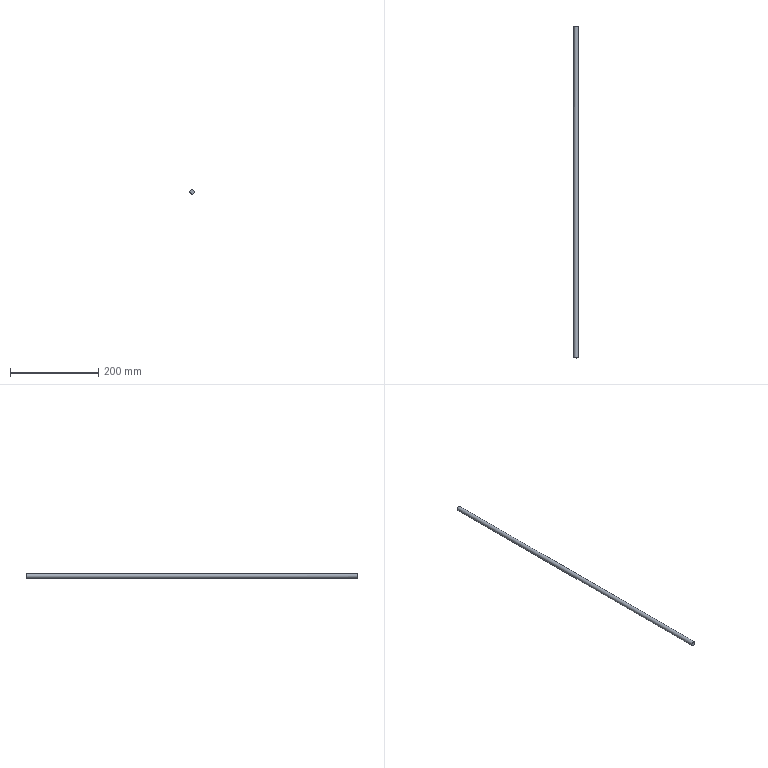Part | NX | features solid 2 | 1 solid | 3 faces | box 10 x 751.5 x 10 mm | volume 59023 mm3 | plane 2 | cylinder 1 | commonest cylinder face diameters 10 x1
STEP:
#1=CARTESIAN_POINT('',(1175.,436.5,-367.));
#2=VERTEX_POINT('',#1);
#3=CARTESIAN_POINT('',(1175.,436.5,-362.));
#4=DIRECTION('',(0.,-1.,0.));
#5=DIRECTION('',(0.,0.,-1.));
#6=AXIS2_PLACEMENT_3D('',#3,#4,#5);
#7=CIRCLE('',#6,5.);
#8=EDGE_CURVE('',#2,#2,#7,.F.);
#9=ORIENTED_EDGE('',*,*,#8,.T.);
#10=EDGE_LOOP('',(#9));
#11=FACE_BOUND('',#10,.T.);
#12=CARTESIAN_POINT('',(1175.,436.5,-362.));
#13=DIRECTION('',(0.,-1.,0.));
#14=DIRECTION('',(0.,0.,1.));
#15=AXIS2_PLACEMENT_3D('',#12,#13,#14);
#16=PLANE('',#15);
#17=ADVANCED_FACE('',(#11),#16,.F.);
#18=CARTESIAN_POINT('',(1170.,-315.,-362.));
#19=VERTEX_POINT('',#18);
#20=CARTESIAN_POINT('',(1175.,-315.,-362.));
#21=DIRECTION('',(0.,1.,0.));
#22=DIRECTION('',(-1.,0.,0.));
#23=AXIS2_PLACEMENT_3D('',#20,#21,#22);
#24=CIRCLE('',#23,5.);
#25=EDGE_CURVE('',#19,#19,#24,.F.);
#26=ORIENTED_EDGE('',*,*,#25,.F.);
#27=EDGE_LOOP('',(#26));
#28=FACE_BOUND('',#27,.T.);
#29=ORIENTED_EDGE('',*,*,#8,.F.);
#30=EDGE_LOOP('',(#29));
#31=FACE_BOUND('',#30,.T.);
#32=CARTESIAN_POINT('',(1175.,-613.5,-362.));
#33=DIRECTION('',(0.,1.,0.));
#34=DIRECTION('',(0.,0.,-1.));
#35=AXIS2_PLACEMENT_3D('',#32,#33,#34);
#36=CYLINDRICAL_SURFACE('',#35,5.);
#37=ADVANCED_FACE('',(#28,#31),#36,.T.);
#38=ORIENTED_EDGE('',*,*,#25,.T.);
#39=EDGE_LOOP('',(#38));
#40=FACE_BOUND('',#39,.T.);
#41=CARTESIAN_POINT('',(1385.,-315.,-350.));
#42=DIRECTION('',(0.,1.,0.));
#43=DIRECTION('',(-1.,0.,0.));
#44=AXIS2_PLACEMENT_3D('',#41,#42,#43);
#45=PLANE('',#44);
#46=ADVANCED_FACE('',(#40),#45,.F.);
#47=CLOSED_SHELL('',(#17,#37,#46));
#48=MANIFOLD_SOLID_BREP('',#47);
#49=(LENGTH_UNIT()NAMED_UNIT(*)SI_UNIT(.MILLI.,.METRE.));
#50=UNCERTAINTY_MEASURE_WITH_UNIT(LENGTH_MEASURE(0.00001),#49,'','');
#51=(NAMED_UNIT(*)PLANE_ANGLE_UNIT()SI_UNIT($,.RADIAN.));
#52=(NAMED_UNIT(*)SI_UNIT($,.STERADIAN.)SOLID_ANGLE_UNIT());
#53=(GEOMETRIC_REPRESENTATION_CONTEXT(3)GLOBAL_UNCERTAINTY_ASSIGNED_CONTEXT((#50))GLOBAL_UNIT_ASSIGNED_CONTEXT((#49,#51,#52))REPRESENTATION_CONTEXT('',''));
#54=ADVANCED_BREP_SHAPE_REPRESENTATION('',(#48),#53);